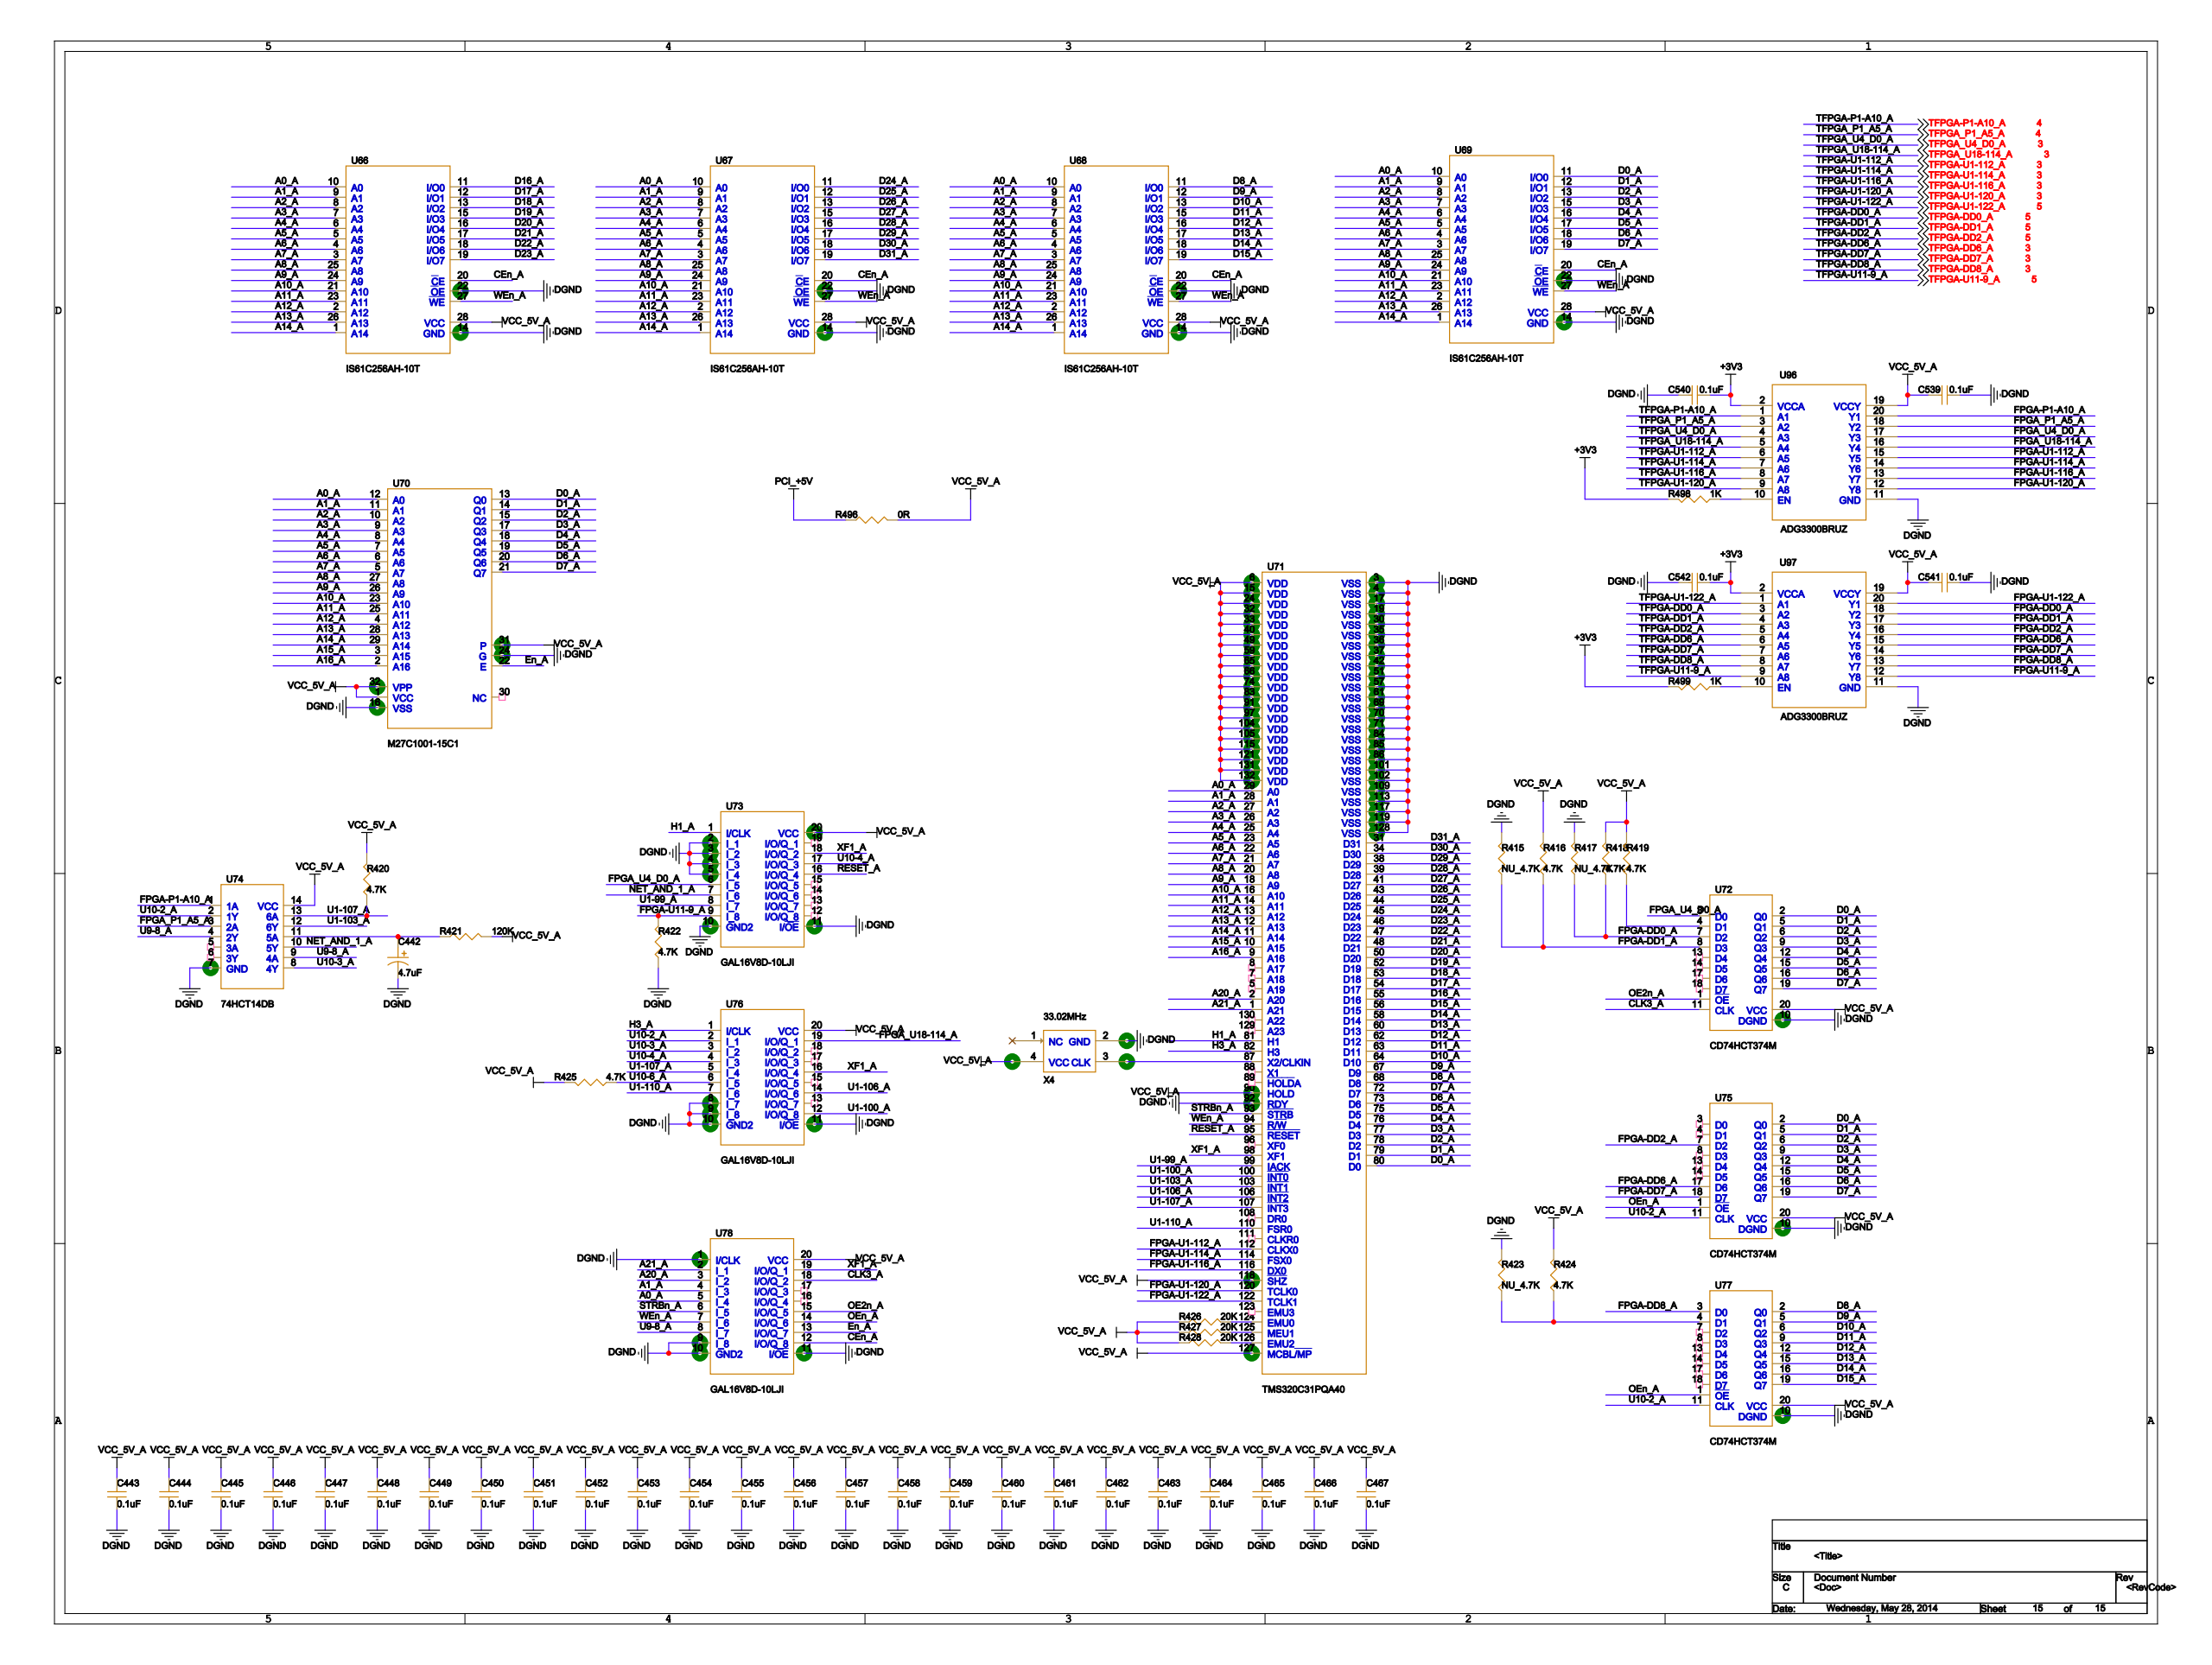Circuit board | Cadence Allegro | 669 parts | 806 nets | one sheet of the schematic
Parts on this sheet (reference | value | footprint):
C442 | 4.7uF | CP3216
C443 | 0.1uF | C0402
C444 | 0.1uF | C0402
C445 | 0.1uF | C0402
C446 | 0.1uF | C0402
C447 | 0.1uF | C0402
C448 | 0.1uF | C0402
C449 | 0.1uF | C0402
C450 | 0.1uF | C0402
C451 | 0.1uF | C0402
C452 | 0.1uF | C0402
C453 | 0.1uF | C0402
C454 | 0.1uF | C0402
C455 | 0.1uF | C0402
C456 | 0.1uF | C0402
C457 | 0.1uF | C0402
C458 | 0.1uF | C0402
C459 | 0.1uF | C0402
C460 | 0.1uF | C0402
C461 | 0.1uF | C0402
C462 | 0.1uF | C0402
C463 | 0.1uF | C0402
C464 | 0.1uF | C0402
C465 | 0.1uF | C0402
C466 | 0.1uF | C0402
C467 | 0.1uF | C0402
C539 | 0.1uF | C0402
C540 | 0.1uF | C0402
C541 | 0.1uF | C0402
C542 | 0.1uF | C0402
R415 | NU_4.7K | R0603
R416 | 4.7K | R0603
R417 | NU_4.7K | R0603
R418 | 4.7K | R0603
R419 | 4.7K | R0603
R420 | 4.7K | R0603
R421 | 120K | R0603
R422 | 4.7K | R0603
R423 | NU_4.7K | R0603
R424 | 4.7K | R0603
R425 | 4.7K | R0603
R426 | 20K | R0603
R427 | 20K | R0603
R428 | 20K | R0603
R496 | 0R | R1210
R498 | 1K | R0603
R499 | 1K | R0603
U66 | IS61C256AH-10T | TSOP28_0P55M_13P4X8M
U67 | IS61C256AH-10T | TSOP28_0P55M_13P4X8M
U68 | IS61C256AH-10T | TSOP28_0P55M_13P4X8M
U69 | IS61C256AH-10T | TSOP28_0P55M_13P4X8M
U70 | M27C1001-15C1 | PLCC32
U71 | TMS320C31PQA40 | QFP132_0P65M_28X28M
U72 | CD74HCT374M | SOIC20_1P27M_10X13M
U73 | GAL16V8D-10LJI | PLCC20
U74 | 74HCT14DB | SSOP14
U75 | CD74HCT374M | SOIC20_1P27M_10X13M
U76 | GAL16V8D-10LJI | PLCC20
U77 | CD74HCT374M | SOIC20_1P27M_10X13M
U78 | GAL16V8D-10LJI | PLCC20
U96 | ADG3300BRUZ | TSSOP20_0P65M_6P4X6P4M
U97 | ADG3300BRUZ | TSSOP20_0P65M_6P4X6P4M
X4 | 33.02MHz | OSC-SMD7050
Nets of these parts (net: part-pin ...):
DGND: C442-2 C443-1 C444-1 C445-1 C446-1 C447-1 C448-1 C449-1 C450-1 C451-1 C452-1 C453-1 C454-1 C455-1 C456-1 C457-1 C458-1 C459-1 C460-1 C461-1 C462-1 C463-1 C464-1 C465-1 C466-1 C467-1 C539-1 C540-2 C541-1 C542-2 R415-2 R417-2 R422-1 R423-2 U72-10 U73-2 U73-3 U73-4 U73-5 U73-10 U73-11 U74-7 U75-10 U76-8 U76-9 U76-10 U76-11 U77-10 U78-1 U78-9 U78-10 U78-11 U96-11 U97-11 X4-2 U66-14 U66-22 U67-14 U67-22 U68-14 U68-22 U69-14 U69-22 U70-16 U70-24 U71-3 U71-4 U71-17 U71-19 U71-30 U71-35 U71-36 U71-37 U71-42 U71-51 U71-57 U71-61 U71-69 U71-70 U71-71 U71-84 U71-85 U71-86 U71-92 U71-101 U71-102 U71-109 U71-113 U71-117 U71-119 U71-128
+3V3: C540-1 C542-1 R498-2 R499-2 U96-2 U97-2
TFPGA-DD6_A: U97-6
TFPGA-U1-112_A: U96-6
TFPGA-U1-114_A: U96-7
TFPGA-U1-116_A: U96-8
TFPGA-DD7_A: U97-7
TFPGA-U1-120_A: U96-9
TFPGA-DD1_A: U97-4
TFPGA-DD0_A: U97-3
TFPGA-DD8_A: U97-8
TFPGA-U1-122_A: U97-1
TFPGA-U11-9_A: U97-9
TFPGA-DD2_A: U97-5
TFPGA_U18-114_A: U96-5
TFPGA_U4_D0_A: U96-4
TFPGA-P1-A10_A: U96-1
TFPGA_P1_A5_A: U96-3
A0_A: U78-5 U66-10 U67-10 U68-10 U69-10 U70-12 U71-29
A1_A: U78-4 U66-9 U67-9 U68-9 U69-9 U70-11 U71-28
A10_A: U66-21 U67-21 U68-21 U69-21 U70-23 U71-16
A11_A: U66-23 U67-23 U68-23 U69-23 U70-25 U71-14
A12_A: U66-2 U67-2 U68-2 U69-2 U70-4 U71-13
A13_A: U66-26 U67-26 U68-26 U69-26 U70-28 U71-12
A14_A: U66-1 U67-1 U68-1 U69-1 U70-29 U71-11
A2_A: U66-8 U67-8 U68-8 U69-8 U70-10 U71-27
A3_A: U66-7 U67-7 U68-7 U69-7 U70-9 U71-26
A4_A: U66-6 U67-6 U68-6 U69-6 U70-8 U71-25
A5_A: U66-5 U67-5 U68-5 U69-5 U70-7 U71-23
A6_A: U66-4 U67-4 U68-4 U69-4 U70-6 U71-22
A7_A: U66-3 U67-3 U68-3 U69-3 U70-5 U71-21
A8_A: U66-25 U67-25 U68-25 U69-25 U70-27 U71-20
A9_A: U66-24 U67-24 U68-24 U69-24 U70-26 U71-18
D16_A: U66-11 U71-55
D17_A: U66-12 U71-54
D18_A: U66-13 U71-53
D19_A: U66-15 U71-52
D20_A: U66-16 U71-50
D21_A: U66-17 U71-48
D22_A: U66-18 U71-47
D23_A: U66-19 U71-46
VCC_5V_A: C443-2 C444-2 C445-2 C446-2 C447-2 C448-2 C449-2 C450-2 C451-2 C452-2 C453-2 C454-2 C455-2 C456-2 C457-2 C458-2 C459-2 C460-2 C461-2 C462-2 C463-2 C464-2 C465-2 C466-2 C467-2 C539-2 C541-2 R416-2 R418-2 R419-2 R420-2 R421-2 R424-2 R425-2 R426-1 R427-1 R428-1 R496-2 U72-20 U73-20 U74-14 U75-20 U76-20 U77-20 U78-20 U96-19 U97-19 X4-4 U66-28 U67-28 U68-28 U69-28 U70-1 U70-31 U70-32 U71-6 U71-15 U71-24 U71-32 U71-33 U71-40 U71-49 U71-59 U71-65 U71-66 U71-74 U71-83 U71-90 U71-91 U71-97 U71-104 U71-105 U71-115 U71-118 U71-121 U71-127 U71-131 U71-132
CEN_A: U78-12 U66-20 U67-20 U68-20 U69-20
WEN_A: U78-7 U66-27 U67-27 U68-27 U69-27 U71-94
D24_A: U67-11 U71-45
D25_A: U67-12 U71-44
D26_A: U67-13 U71-43
D27_A: U67-15 U71-41
D28_A: U67-16 U71-39
D29_A: U67-17 U71-38
D30_A: U67-18 U71-34
D31_A: U67-19 U71-31
D8_A: U77-2 U68-11 U71-68
D9_A: U77-5 U68-12 U71-67
D10_A: U77-6 U68-13 U71-64
D11_A: U77-9 U68-15 U71-63
D12_A: U77-12 U68-16 U71-62
D13_A: U77-15 U68-17 U71-60
D14_A: U77-16 U68-18 U71-58
D15_A: U77-19 U68-19 U71-56
D0_A: U72-2 U75-2 U69-11 U70-13 U71-80
D1_A: U72-5 U75-5 U69-12 U70-14 U71-79
D2_A: U72-6 U75-6 U69-13 U70-15 U71-78
D3_A: U72-9 U75-9 U69-15 U70-17 U71-77
D4_A: U72-12 U75-12 U69-16 U70-18 U71-76
D5_A: U72-15 U75-15 U69-17 U70-19 U71-75
D6_A: U72-16 U75-16 U69-18 U70-20 U71-73
D7_A: U72-19 U75-19 U69-19 U70-21 U71-72
A15_A: U70-3 U71-10
A16_A: U70-2 U71-9
EN_A: U78-13 U70-22
A20_A: U78-3 U71-2
A21_A: U78-2 U71-1
FPGA-U1-112_A: U96-15 U71-112
FPGA-U1-116_A: U96-13 U71-116
N16313834: R426-2 U71-124
N16313842: R428-2 U71-126
U1-110_A: U76-7 U71-110
FPGA-U1-114_A: U96-14 U71-114
H1_A: U73-1 U71-81
H3_A: U76-1 U71-82
U1-99_A: U73-8 U71-99
N16313846: R427-2 U71-125
FPGA-U1-120_A: U96-12 U71-120
FPGA-U1-122_A: U97-20 U71-122
N16313988: X4-3 U71-87
XF1_A: U73-18 U76-16 U78-19 U71-98
U1-100_A: U76-12 U71-100
U1-103_A: U74-12 U71-103
U1-106_A: U76-14 U71-106
U1-107_A: R420-1 U74-13 U76-5 U71-107
RESET_A: U73-16 U71-95
STRBN_A: U78-6 U71-93
CLK3_A: U72-11 U78-18
FPGA_U4_D0_A: U72-3 U73-6 U96-17
N16310932: R419-1 U72-4
FPGA-DD0_A: R417-1 R418-1 U72-7 U97-18
FPGA-DD1_A: R415-1 R416-1 U72-8 U97-17
OE2N_A: U72-1 U78-15
U10-2_A: U74-2 U75-11 U76-2 U77-11
FPGA-DD2_A: U75-7 U97-16
FPGA-DD6_A: U75-17 U97-15
FPGA-DD7_A: U75-18 U97-14
OEN_A: U75-1 U77-1 U78-14
FPGA-DD8_A: U77-3 U97-13
N16311742: R423-1 R424-1 U77-4
FPGA-P1-A10_A: U74-1 U96-20
FPGA_P1_A5_A: U74-3 U96-18
U9-8_A: U74-4 U74-9 U78-8
U10-3_A: U74-8 U76-3
N16312392: C442-1 R421-1 U74-11
NET_AND_1_A: U73-7 U74-10
U10-4_A: U73-17 U76-4
FPGA-U11-9_A: R422-2 U73-9 U97-12
FPGA_U18-114_A: U76-19 U96-16
U10-6_A: R425-1 U76-6
N61241770: R498-1 U96-10
N61241864: R499-1 U97-10
PCI_+5V: R496-1